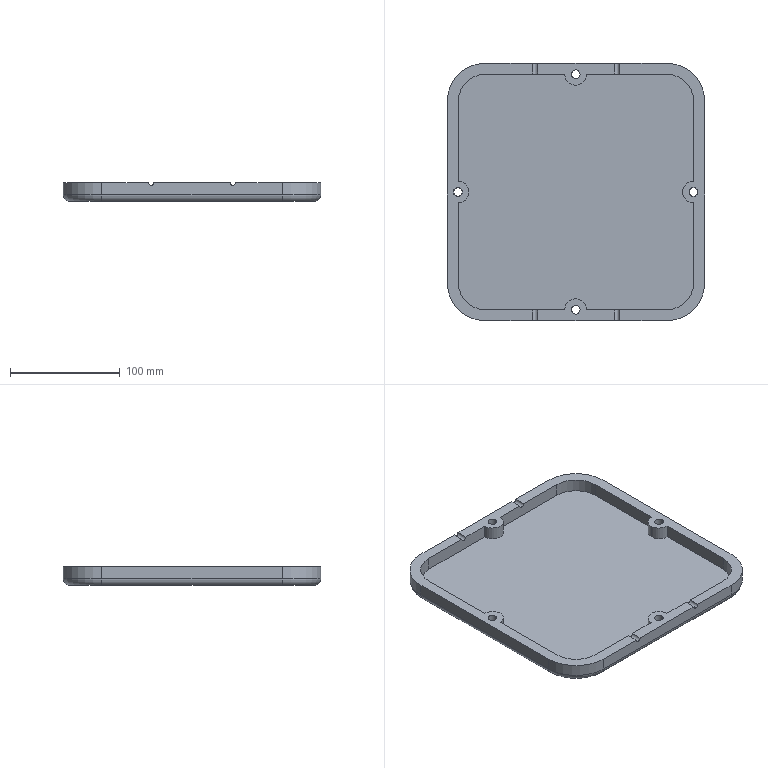Part | SolidWorks | features ICE 2, Extrusion 1, Fillet 1 | 1 solid | 69 faces | box 235 x 235 x 17 mm | volume 369692 mm3 | cylinder 39 | plane 26 | torus 4 | commonest cylinder face diameters 8 x16 20 x7 5 x4 12 x4 50 x4 70 x4